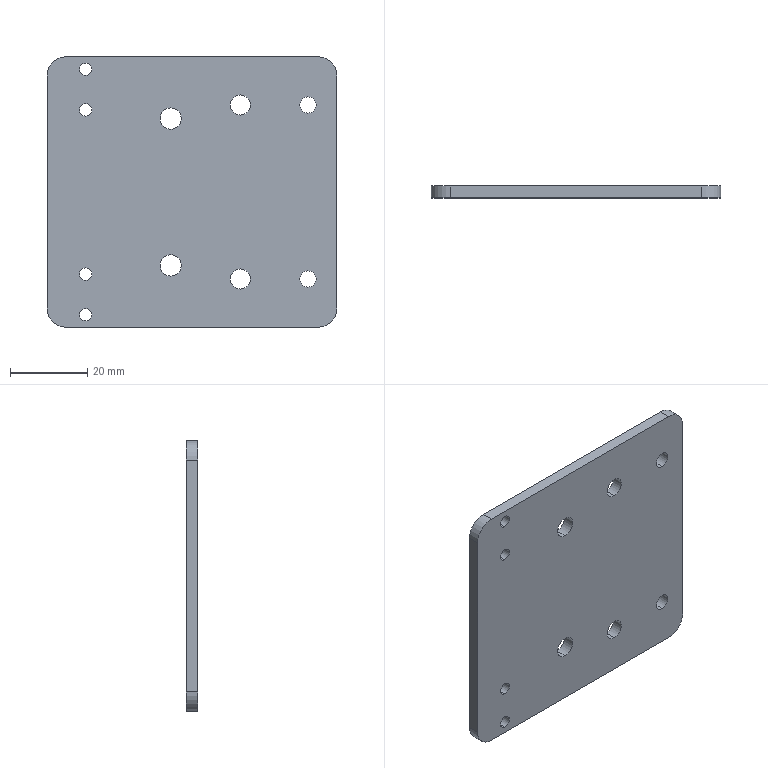Part | SolidWorks | features BaseBody 1 | 1 solid | 30 faces | box 75 x 3 x 70 mm | volume 15236 mm3 | cylinder 24 | plane 6 | commonest cylinder face diameters 3.2 x8 4.2 x4 5.2 x4 5.5 x4 10 x4
STEP:
#1=CARTESIAN_POINT('',(-7.5,3.,25.1));
#2=VERTEX_POINT('',#1);
#3=CARTESIAN_POINT('',(-7.5,3.,19.9));
#4=VERTEX_POINT('',#3);
#5=CARTESIAN_POINT('',(-7.5,3.,22.5));
#6=DIRECTION('',(0.,-1.,0.));
#7=DIRECTION('',(0.,0.,-1.));
#8=AXIS2_PLACEMENT_3D('',#5,#6,#7);
#9=CIRCLE('',#8,2.6);
#10=EDGE_CURVE('',#2,#4,#9,.T.);
#11=ORIENTED_EDGE('',*,*,#10,.F.);
#12=CARTESIAN_POINT('',(-7.5,0.,25.1));
#13=VERTEX_POINT('',#12);
#14=CARTESIAN_POINT('',(-7.5,3.,25.1));
#15=DIRECTION('',(0.,-1.,0.));
#16=VECTOR('',#15,1000.);
#17=LINE('',#14,#16);
#18=EDGE_CURVE('',#2,#13,#17,.T.);
#19=ORIENTED_EDGE('',*,*,#18,.T.);
#20=CARTESIAN_POINT('',(-7.5,0.,19.9));
#21=VERTEX_POINT('',#20);
#22=CARTESIAN_POINT('',(-7.5,0.,22.5));
#23=DIRECTION('',(0.,1.,0.));
#24=DIRECTION('',(0.,0.,-1.));
#25=AXIS2_PLACEMENT_3D('',#22,#23,#24);
#26=CIRCLE('',#25,2.6);
#27=EDGE_CURVE('',#21,#13,#26,.T.);
#28=ORIENTED_EDGE('',*,*,#27,.F.);
#29=CARTESIAN_POINT('',(-7.5,3.,19.9));
#30=DIRECTION('',(0.,-1.,0.));
#31=VECTOR('',#30,1000.);
#32=LINE('',#29,#31);
#33=EDGE_CURVE('',#4,#21,#32,.T.);
#34=ORIENTED_EDGE('',*,*,#33,.F.);
#35=EDGE_LOOP('',(#11,#19,#28,#34));
#36=FACE_OUTER_BOUND('',#35,.T.);
#37=CARTESIAN_POINT('',(-7.5,3.,22.5));
#38=DIRECTION('',(0.,-1.,0.));
#39=DIRECTION('',(0.,0.,-1.));
#40=AXIS2_PLACEMENT_3D('',#37,#38,#39);
#41=CYLINDRICAL_SURFACE('',#40,2.6);
#42=ADVANCED_FACE('',(#36),#41,.F.);
#43=CARTESIAN_POINT('',(-7.5,3.,-19.9));
#44=VERTEX_POINT('',#43);
#45=CARTESIAN_POINT('',(-7.5,3.,-25.1));
#46=VERTEX_POINT('',#45);
#47=CARTESIAN_POINT('',(-7.5,3.,-22.5));
#48=DIRECTION('',(0.,-1.,0.));
#49=DIRECTION('',(0.,0.,-1.));
#50=AXIS2_PLACEMENT_3D('',#47,#48,#49);
#51=CIRCLE('',#50,2.6);
#52=EDGE_CURVE('',#44,#46,#51,.T.);
#53=ORIENTED_EDGE('',*,*,#52,.F.);
#54=CARTESIAN_POINT('',(-7.5,0.,-19.9));
#55=VERTEX_POINT('',#54);
#56=CARTESIAN_POINT('',(-7.5,3.,-19.9));
#57=DIRECTION('',(0.,-1.,0.));
#58=VECTOR('',#57,1000.);
#59=LINE('',#56,#58);
#60=EDGE_CURVE('',#44,#55,#59,.T.);
#61=ORIENTED_EDGE('',*,*,#60,.T.);
#62=CARTESIAN_POINT('',(-7.5,0.,-25.1));
#63=VERTEX_POINT('',#62);
#64=CARTESIAN_POINT('',(-7.5,0.,-22.5));
#65=DIRECTION('',(0.,1.,0.));
#66=DIRECTION('',(0.,0.,-1.));
#67=AXIS2_PLACEMENT_3D('',#64,#65,#66);
#68=CIRCLE('',#67,2.6);
#69=EDGE_CURVE('',#63,#55,#68,.T.);
#70=ORIENTED_EDGE('',*,*,#69,.F.);
#71=CARTESIAN_POINT('',(-7.5,3.,-25.1));
#72=DIRECTION('',(0.,-1.,0.));
#73=VECTOR('',#72,1000.);
#74=LINE('',#71,#73);
#75=EDGE_CURVE('',#46,#63,#74,.T.);
#76=ORIENTED_EDGE('',*,*,#75,.F.);
#77=EDGE_LOOP('',(#53,#61,#70,#76));
#78=FACE_OUTER_BOUND('',#77,.T.);
#79=CARTESIAN_POINT('',(-7.5,3.,-22.5));
#80=DIRECTION('',(0.,-1.,0.));
#81=DIRECTION('',(0.,0.,-1.));
#82=AXIS2_PLACEMENT_3D('',#79,#80,#81);
#83=CYLINDRICAL_SURFACE('',#82,2.6);
#84=ADVANCED_FACE('',(#78),#83,.F.);
#85=CARTESIAN_POINT('',(10.,0.,-24.6));
#86=VERTEX_POINT('',#85);
#87=CARTESIAN_POINT('',(10.,0.,-20.4));
#88=VERTEX_POINT('',#87);
#89=CARTESIAN_POINT('',(10.,0.,-22.5));
#90=DIRECTION('',(0.,1.,0.));
#91=DIRECTION('',(0.,0.,1.));
#92=AXIS2_PLACEMENT_3D('',#89,#90,#91);
#93=CIRCLE('',#92,2.1);
#94=EDGE_CURVE('',#86,#88,#93,.T.);
#95=ORIENTED_EDGE('',*,*,#94,.F.);
#96=CARTESIAN_POINT('',(10.,3.,-24.6));
#97=VERTEX_POINT('',#96);
#98=CARTESIAN_POINT('',(10.,0.,-24.6));
#99=DIRECTION('',(0.,1.,0.));
#100=VECTOR('',#99,1000.);
#101=LINE('',#98,#100);
#102=EDGE_CURVE('',#86,#97,#101,.T.);
#103=ORIENTED_EDGE('',*,*,#102,.T.);
#104=CARTESIAN_POINT('',(10.,3.,-20.4));
#105=VERTEX_POINT('',#104);
#106=CARTESIAN_POINT('',(10.,3.,-22.5));
#107=DIRECTION('',(0.,-1.,0.));
#108=DIRECTION('',(0.,0.,1.));
#109=AXIS2_PLACEMENT_3D('',#106,#107,#108);
#110=CIRCLE('',#109,2.1);
#111=EDGE_CURVE('',#105,#97,#110,.T.);
#112=ORIENTED_EDGE('',*,*,#111,.F.);
#113=CARTESIAN_POINT('',(10.,0.,-20.4));
#114=DIRECTION('',(0.,1.,0.));
#115=VECTOR('',#114,1000.);
#116=LINE('',#113,#115);
#117=EDGE_CURVE('',#88,#105,#116,.T.);
#118=ORIENTED_EDGE('',*,*,#117,.F.);
#119=EDGE_LOOP('',(#95,#103,#112,#118));
#120=FACE_OUTER_BOUND('',#119,.T.);
#121=CARTESIAN_POINT('',(10.,0.,-22.5));
#122=DIRECTION('',(0.,1.,0.));
#123=DIRECTION('',(0.,0.,1.));
#124=AXIS2_PLACEMENT_3D('',#121,#122,#123);
#125=CYLINDRICAL_SURFACE('',#124,2.1);
#126=ADVANCED_FACE('',(#120),#125,.F.);
#127=CARTESIAN_POINT('',(10.,0.,20.4));
#128=VERTEX_POINT('',#127);
#129=CARTESIAN_POINT('',(10.,0.,24.6));
#130=VERTEX_POINT('',#129);
#131=CARTESIAN_POINT('',(10.,0.,22.5));
#132=DIRECTION('',(0.,1.,0.));
#133=DIRECTION('',(0.,0.,1.));
#134=AXIS2_PLACEMENT_3D('',#131,#132,#133);
#135=CIRCLE('',#134,2.1);
#136=EDGE_CURVE('',#128,#130,#135,.T.);
#137=ORIENTED_EDGE('',*,*,#136,.F.);
#138=CARTESIAN_POINT('',(10.,3.,20.4));
#139=VERTEX_POINT('',#138);
#140=CARTESIAN_POINT('',(10.,0.,20.4));
#141=DIRECTION('',(0.,1.,0.));
#142=VECTOR('',#141,1000.);
#143=LINE('',#140,#142);
#144=EDGE_CURVE('',#128,#139,#143,.T.);
#145=ORIENTED_EDGE('',*,*,#144,.T.);
#146=CARTESIAN_POINT('',(10.,3.,24.6));
#147=VERTEX_POINT('',#146);
#148=CARTESIAN_POINT('',(10.,3.,22.5));
#149=DIRECTION('',(0.,-1.,0.));
#150=DIRECTION('',(0.,0.,1.));
#151=AXIS2_PLACEMENT_3D('',#148,#149,#150);
#152=CIRCLE('',#151,2.1);
#153=EDGE_CURVE('',#147,#139,#152,.T.);
#154=ORIENTED_EDGE('',*,*,#153,.F.);
#155=CARTESIAN_POINT('',(10.,0.,24.6));
#156=DIRECTION('',(0.,1.,0.));
#157=VECTOR('',#156,1000.);
#158=LINE('',#155,#157);
#159=EDGE_CURVE('',#130,#147,#158,.T.);
#160=ORIENTED_EDGE('',*,*,#159,.F.);
#161=EDGE_LOOP('',(#137,#145,#154,#160));
#162=FACE_OUTER_BOUND('',#161,.T.);
#163=CARTESIAN_POINT('',(10.,0.,22.5));
#164=DIRECTION('',(0.,1.,0.));
#165=DIRECTION('',(0.,0.,1.));
#166=AXIS2_PLACEMENT_3D('',#163,#164,#165);
#167=CYLINDRICAL_SURFACE('',#166,2.1);
#168=ADVANCED_FACE('',(#162),#167,.F.);
#169=CARTESIAN_POINT('',(-47.5,3.,22.85));
#170=VERTEX_POINT('',#169);
#171=CARTESIAN_POINT('',(-47.5,3.,19.65));
#172=VERTEX_POINT('',#171);
#173=CARTESIAN_POINT('',(-47.5,3.,21.25));
#174=DIRECTION('',(0.,-1.,0.));
#175=DIRECTION('',(0.,0.,-1.));
#176=AXIS2_PLACEMENT_3D('',#173,#174,#175);
#177=CIRCLE('',#176,1.6);
#178=EDGE_CURVE('',#170,#172,#177,.T.);
#179=ORIENTED_EDGE('',*,*,#178,.F.);
#180=CARTESIAN_POINT('',(-47.5,0.,22.85));
#181=VERTEX_POINT('',#180);
#182=CARTESIAN_POINT('',(-47.5,3.,22.85));
#183=DIRECTION('',(0.,-1.,0.));
#184=VECTOR('',#183,1000.);
#185=LINE('',#182,#184);
#186=EDGE_CURVE('',#170,#181,#185,.T.);
#187=ORIENTED_EDGE('',*,*,#186,.T.);
#188=CARTESIAN_POINT('',(-47.5,0.,19.65));
#189=VERTEX_POINT('',#188);
#190=CARTESIAN_POINT('',(-47.5,0.,21.25));
#191=DIRECTION('',(0.,1.,0.));
#192=DIRECTION('',(0.,0.,-1.));
#193=AXIS2_PLACEMENT_3D('',#190,#191,#192);
#194=CIRCLE('',#193,1.6);
#195=EDGE_CURVE('',#189,#181,#194,.T.);
#196=ORIENTED_EDGE('',*,*,#195,.F.);
#197=CARTESIAN_POINT('',(-47.5,3.,19.65));
#198=DIRECTION('',(0.,-1.,0.));
#199=VECTOR('',#198,1000.);
#200=LINE('',#197,#199);
#201=EDGE_CURVE('',#172,#189,#200,.T.);
#202=ORIENTED_EDGE('',*,*,#201,.F.);
#203=EDGE_LOOP('',(#179,#187,#196,#202));
#204=FACE_OUTER_BOUND('',#203,.T.);
#205=CARTESIAN_POINT('',(-47.5,3.,21.25));
#206=DIRECTION('',(0.,-1.,0.));
#207=DIRECTION('',(0.,0.,-1.));
#208=AXIS2_PLACEMENT_3D('',#205,#206,#207);
#209=CYLINDRICAL_SURFACE('',#208,1.6);
#210=ADVANCED_FACE('',(#204),#209,.F.);
#211=CARTESIAN_POINT('',(-47.5,3.,33.35));
#212=VERTEX_POINT('',#211);
#213=CARTESIAN_POINT('',(-47.5,3.,30.15));
#214=VERTEX_POINT('',#213);
#215=CARTESIAN_POINT('',(-47.5,3.,31.75));
#216=DIRECTION('',(0.,-1.,0.));
#217=DIRECTION('',(0.,0.,-1.));
#218=AXIS2_PLACEMENT_3D('',#215,#216,#217);
#219=CIRCLE('',#218,1.6);
#220=EDGE_CURVE('',#212,#214,#219,.T.);
#221=ORIENTED_EDGE('',*,*,#220,.F.);
#222=CARTESIAN_POINT('',(-47.5,0.,33.35));
#223=VERTEX_POINT('',#222);
#224=CARTESIAN_POINT('',(-47.5,3.,33.35));
#225=DIRECTION('',(0.,-1.,0.));
#226=VECTOR('',#225,1000.);
#227=LINE('',#224,#226);
#228=EDGE_CURVE('',#212,#223,#227,.T.);
#229=ORIENTED_EDGE('',*,*,#228,.T.);
#230=CARTESIAN_POINT('',(-47.5,0.,30.15));
#231=VERTEX_POINT('',#230);
#232=CARTESIAN_POINT('',(-47.5,0.,31.75));
#233=DIRECTION('',(0.,1.,0.));
#234=DIRECTION('',(0.,0.,-1.));
#235=AXIS2_PLACEMENT_3D('',#232,#233,#234);
#236=CIRCLE('',#235,1.6);
#237=EDGE_CURVE('',#231,#223,#236,.T.);
#238=ORIENTED_EDGE('',*,*,#237,.F.);
#239=CARTESIAN_POINT('',(-47.5,3.,30.15));
#240=DIRECTION('',(0.,-1.,0.));
#241=VECTOR('',#240,1000.);
#242=LINE('',#239,#241);
#243=EDGE_CURVE('',#214,#231,#242,.T.);
#244=ORIENTED_EDGE('',*,*,#243,.F.);
#245=EDGE_LOOP('',(#221,#229,#238,#244));
#246=FACE_OUTER_BOUND('',#245,.T.);
#247=CARTESIAN_POINT('',(-47.5,3.,31.75));
#248=DIRECTION('',(0.,-1.,0.));
#249=DIRECTION('',(0.,0.,-1.));
#250=AXIS2_PLACEMENT_3D('',#247,#248,#249);
#251=CYLINDRICAL_SURFACE('',#250,1.6);
#252=ADVANCED_FACE('',(#246),#251,.F.);
#253=CARTESIAN_POINT('',(-47.5,3.,-19.65));
#254=VERTEX_POINT('',#253);
#255=CARTESIAN_POINT('',(-47.5,3.,-22.85));
#256=VERTEX_POINT('',#255);
#257=CARTESIAN_POINT('',(-47.5,3.,-21.25));
#258=DIRECTION('',(0.,-1.,0.));
#259=DIRECTION('',(0.,0.,-1.));
#260=AXIS2_PLACEMENT_3D('',#257,#258,#259);
#261=CIRCLE('',#260,1.6);
#262=EDGE_CURVE('',#254,#256,#261,.T.);
#263=ORIENTED_EDGE('',*,*,#262,.F.);
#264=CARTESIAN_POINT('',(-47.5,0.,-19.65));
#265=VERTEX_POINT('',#264);
#266=CARTESIAN_POINT('',(-47.5,3.,-19.65));
#267=DIRECTION('',(0.,-1.,0.));
#268=VECTOR('',#267,1000.);
#269=LINE('',#266,#268);
#270=EDGE_CURVE('',#254,#265,#269,.T.);
#271=ORIENTED_EDGE('',*,*,#270,.T.);
#272=CARTESIAN_POINT('',(-47.5,0.,-22.85));
#273=VERTEX_POINT('',#272);
#274=CARTESIAN_POINT('',(-47.5,0.,-21.25));
#275=DIRECTION('',(0.,1.,0.));
#276=DIRECTION('',(0.,0.,-1.));
#277=AXIS2_PLACEMENT_3D('',#274,#275,#276);
#278=CIRCLE('',#277,1.6);
#279=EDGE_CURVE('',#273,#265,#278,.T.);
#280=ORIENTED_EDGE('',*,*,#279,.F.);
#281=CARTESIAN_POINT('',(-47.5,3.,-22.85));
#282=DIRECTION('',(0.,-1.,0.));
#283=VECTOR('',#282,1000.);
#284=LINE('',#281,#283);
#285=EDGE_CURVE('',#256,#273,#284,.T.);
#286=ORIENTED_EDGE('',*,*,#285,.F.);
#287=EDGE_LOOP('',(#263,#271,#280,#286));
#288=FACE_OUTER_BOUND('',#287,.T.);
#289=CARTESIAN_POINT('',(-47.5,3.,-21.25));
#290=DIRECTION('',(0.,-1.,0.));
#291=DIRECTION('',(0.,0.,-1.));
#292=AXIS2_PLACEMENT_3D('',#289,#290,#291);
#293=CYLINDRICAL_SURFACE('',#292,1.6);
#294=ADVANCED_FACE('',(#288),#293,.F.);
#295=CARTESIAN_POINT('',(-47.5,3.,-30.15));
#296=VERTEX_POINT('',#295);
#297=CARTESIAN_POINT('',(-47.5,3.,-33.35));
#298=VERTEX_POINT('',#297);
#299=CARTESIAN_POINT('',(-47.5,3.,-31.75));
#300=DIRECTION('',(0.,-1.,0.));
#301=DIRECTION('',(0.,0.,-1.));
#302=AXIS2_PLACEMENT_3D('',#299,#300,#301);
#303=CIRCLE('',#302,1.6);
#304=EDGE_CURVE('',#296,#298,#303,.T.);
#305=ORIENTED_EDGE('',*,*,#304,.F.);
#306=CARTESIAN_POINT('',(-47.5,0.,-30.15));
#307=VERTEX_POINT('',#306);
#308=CARTESIAN_POINT('',(-47.5,3.,-30.15));
#309=DIRECTION('',(0.,-1.,0.));
#310=VECTOR('',#309,1000.);
#311=LINE('',#308,#310);
#312=EDGE_CURVE('',#296,#307,#311,.T.);
#313=ORIENTED_EDGE('',*,*,#312,.T.);
#314=CARTESIAN_POINT('',(-47.5,0.,-33.35));
#315=VERTEX_POINT('',#314);
#316=CARTESIAN_POINT('',(-47.5,0.,-31.75));
#317=DIRECTION('',(0.,1.,0.));
#318=DIRECTION('',(0.,0.,-1.));
#319=AXIS2_PLACEMENT_3D('',#316,#317,#318);
#320=CIRCLE('',#319,1.6);
#321=EDGE_CURVE('',#315,#307,#320,.T.);
#322=ORIENTED_EDGE('',*,*,#321,.F.);
#323=CARTESIAN_POINT('',(-47.5,3.,-33.35));
#324=DIRECTION('',(0.,-1.,0.));
#325=VECTOR('',#324,1000.);
#326=LINE('',#323,#325);
#327=EDGE_CURVE('',#298,#315,#326,.T.);
#328=ORIENTED_EDGE('',*,*,#327,.F.);
#329=EDGE_LOOP('',(#305,#313,#322,#328));
#330=FACE_OUTER_BOUND('',#329,.T.);
#331=CARTESIAN_POINT('',(-47.5,3.,-31.75));
#332=DIRECTION('',(0.,-1.,0.));
#333=DIRECTION('',(0.,0.,-1.));
#334=AXIS2_PLACEMENT_3D('',#331,#332,#333);
#335=CYLINDRICAL_SURFACE('',#334,1.6);
#336=ADVANCED_FACE('',(#330),#335,.F.);
#337=CARTESIAN_POINT('',(-25.5,0.,-21.75));
#338=VERTEX_POINT('',#337);
#339=CARTESIAN_POINT('',(-25.5,0.,-16.25));
#340=VERTEX_POINT('',#339);
#341=CARTESIAN_POINT('',(-25.5,0.,-19.));
#342=DIRECTION('',(0.,1.,0.));
#343=DIRECTION('',(0.,0.,1.));
#344=AXIS2_PLACEMENT_3D('',#341,#342,#343);
#345=CIRCLE('',#344,2.75);
#346=EDGE_CURVE('',#338,#340,#345,.T.);
#347=ORIENTED_EDGE('',*,*,#346,.F.);
#348=CARTESIAN_POINT('',(-25.5,3.,-21.75));
#349=VERTEX_POINT('',#348);
#350=CARTESIAN_POINT('',(-25.5,-2.5,-21.75));
#351=DIRECTION('',(0.,1.,0.));
#352=VECTOR('',#351,1000.);
#353=LINE('',#350,#352);
#354=EDGE_CURVE('',#338,#349,#353,.T.);
#355=ORIENTED_EDGE('',*,*,#354,.T.);
#356=CARTESIAN_POINT('',(-25.5,3.,-16.25));
#357=VERTEX_POINT('',#356);
#358=CARTESIAN_POINT('',(-25.5,3.,-19.));
#359=DIRECTION('',(0.,-1.,0.));
#360=DIRECTION('',(0.,0.,1.));
#361=AXIS2_PLACEMENT_3D('',#358,#359,#360);
#362=CIRCLE('',#361,2.75);
#363=EDGE_CURVE('',#357,#349,#362,.T.);
#364=ORIENTED_EDGE('',*,*,#363,.F.);
#365=CARTESIAN_POINT('',(-25.5,-2.5,-16.25));
#366=DIRECTION('',(0.,1.,0.));
#367=VECTOR('',#366,1000.);
#368=LINE('',#365,#367);
#369=EDGE_CURVE('',#340,#357,#368,.T.);
#370=ORIENTED_EDGE('',*,*,#369,.F.);
#371=EDGE_LOOP('',(#347,#355,#364,#370));
#372=FACE_OUTER_BOUND('',#371,.T.);
#373=CARTESIAN_POINT('',(-25.5,-2.5,-19.));
#374=DIRECTION('',(0.,1.,0.));
#375=DIRECTION('',(0.,0.,1.));
#376=AXIS2_PLACEMENT_3D('',#373,#374,#375);
#377=CYLINDRICAL_SURFACE('',#376,2.75);
#378=ADVANCED_FACE('',(#372),#377,.F.);
#379=CARTESIAN_POINT('',(-25.5,0.,16.25));
#380=VERTEX_POINT('',#379);
#381=CARTESIAN_POINT('',(-25.5,0.,21.75));
#382=VERTEX_POINT('',#381);
#383=CARTESIAN_POINT('',(-25.5,0.,19.));
#384=DIRECTION('',(0.,1.,0.));
#385=DIRECTION('',(0.,0.,1.));
#386=AXIS2_PLACEMENT_3D('',#383,#384,#385);
#387=CIRCLE('',#386,2.75);
#388=EDGE_CURVE('',#380,#382,#387,.T.);
#389=ORIENTED_EDGE('',*,*,#388,.F.);
#390=CARTESIAN_POINT('',(-25.5,3.,16.25));
#391=VERTEX_POINT('',#390);
#392=CARTESIAN_POINT('',(-25.5,-2.5,16.25));
#393=DIRECTION('',(0.,1.,0.));
#394=VECTOR('',#393,1000.);
#395=LINE('',#392,#394);
#396=EDGE_CURVE('',#380,#391,#395,.T.);
#397=ORIENTED_EDGE('',*,*,#396,.T.);
#398=CARTESIAN_POINT('',(-25.5,3.,21.75));
#399=VERTEX_POINT('',#398);
#400=CARTESIAN_POINT('',(-25.5,3.,19.));
#401=DIRECTION('',(0.,-1.,0.));
#402=DIRECTION('',(0.,0.,1.));
#403=AXIS2_PLACEMENT_3D('',#400,#401,#402);
#404=CIRCLE('',#403,2.75);
#405=EDGE_CURVE('',#399,#391,#404,.T.);
#406=ORIENTED_EDGE('',*,*,#405,.F.);
#407=CARTESIAN_POINT('',(-25.5,-2.5,21.75));
#408=DIRECTION('',(0.,1.,0.));
#409=VECTOR('',#408,1000.);
#410=LINE('',#407,#409);
#411=EDGE_CURVE('',#382,#399,#410,.T.);
#412=ORIENTED_EDGE('',*,*,#411,.F.);
#413=EDGE_LOOP('',(#389,#397,#406,#412));
#414=FACE_OUTER_BOUND('',#413,.T.);
#415=CARTESIAN_POINT('',(-25.5,-2.5,19.));
#416=DIRECTION('',(0.,1.,0.));
#417=DIRECTION('',(0.,0.,1.));
#418=AXIS2_PLACEMENT_3D('',#415,#416,#417);
#419=CYLINDRICAL_SURFACE('',#418,2.75);
#420=ADVANCED_FACE('',(#414),#419,.F.);
#421=ORIENTED_EDGE('',*,*,#27,.T.);
#422=CARTESIAN_POINT('',(-7.5,0.,22.5));
#423=DIRECTION('',(0.,1.,0.));
#424=DIRECTION('',(0.,0.,-1.));
#425=AXIS2_PLACEMENT_3D('',#422,#423,#424);
#426=CIRCLE('',#425,2.6);
#427=EDGE_CURVE('',#13,#21,#426,.T.);
#428=ORIENTED_EDGE('',*,*,#427,.T.);
#429=EDGE_LOOP('',(#421,#428));
#430=FACE_BOUND('',#429,.T.);
#431=ORIENTED_EDGE('',*,*,#69,.T.);
#432=CARTESIAN_POINT('',(-7.5,0.,-22.5));
#433=DIRECTION('',(0.,1.,0.));
#434=DIRECTION('',(0.,0.,-1.));
#435=AXIS2_PLACEMENT_3D('',#432,#433,#434);
#436=CIRCLE('',#435,2.6);
#437=EDGE_CURVE('',#55,#63,#436,.T.);
#438=ORIENTED_EDGE('',*,*,#437,.T.);
#439=EDGE_LOOP('',(#431,#438));
#440=FACE_BOUND('',#439,.T.);
#441=CARTESIAN_POINT('',(10.,0.,-22.5));
#442=DIRECTION('',(0.,1.,0.));
#443=DIRECTION('',(0.,0.,1.));
#444=AXIS2_PLACEMENT_3D('',#441,#442,#443);
#445=CIRCLE('',#444,2.1);
#446=EDGE_CURVE('',#88,#86,#445,.T.);
#447=ORIENTED_EDGE('',*,*,#446,.T.);
#448=ORIENTED_EDGE('',*,*,#94,.T.);
#449=EDGE_LOOP('',(#447,#448));
#450=FACE_BOUND('',#449,.T.);
#451=CARTESIAN_POINT('',(10.,0.,22.5));
#452=DIRECTION('',(0.,1.,0.));
#453=DIRECTION('',(0.,0.,1.));
#454=AXIS2_PLACEMENT_3D('',#451,#452,#453);
#455=CIRCLE('',#454,2.1);
#456=EDGE_CURVE('',#130,#128,#455,.T.);
#457=ORIENTED_EDGE('',*,*,#456,.T.);
#458=ORIENTED_EDGE('',*,*,#136,.T.);
#459=EDGE_LOOP('',(#457,#458));
#460=FACE_BOUND('',#459,.T.);
#461=ORIENTED_EDGE('',*,*,#195,.T.);
#462=CARTESIAN_POINT('',(-47.5,0.,21.25));
#463=DIRECTION('',(0.,1.,0.));
#464=DIRECTION('',(0.,0.,-1.));
#465=AXIS2_PLACEMENT_3D('',#462,#463,#464);
#466=CIRCLE('',#465,1.6);
#467=EDGE_CURVE('',#181,#189,#466,.T.);
#468=ORIENTED_EDGE('',*,*,#467,.T.);
#469=EDGE_LOOP('',(#461,#468));
#470=FACE_BOUND('',#469,.T.);
#471=ORIENTED_EDGE('',*,*,#237,.T.);
#472=CARTESIAN_POINT('',(-47.5,0.,31.75));
#473=DIRECTION('',(0.,1.,0.));
#474=DIRECTION('',(0.,0.,-1.));
#475=AXIS2_PLACEMENT_3D('',#472,#473,#474);
#476=CIRCLE('',#475,1.6);
#477=EDGE_CURVE('',#223,#231,#476,.T.);
#478=ORIENTED_EDGE('',*,*,#477,.T.);
#479=EDGE_LOOP('',(#471,#478));
#480=FACE_BOUND('',#479,.T.);
#481=ORIENTED_EDGE('',*,*,#279,.T.);
#482=CARTESIAN_POINT('',(-47.5,0.,-21.25));
#483=DIRECTION('',(0.,1.,0.));
#484=DIRECTION('',(0.,0.,-1.));
#485=AXIS2_PLACEMENT_3D('',#482,#483,#484);
#486=CIRCLE('',#485,1.6);
#487=EDGE_CURVE('',#265,#273,#486,.T.);
#488=ORIENTED_EDGE('',*,*,#487,.T.);
#489=EDGE_LOOP('',(#481,#488));
#490=FACE_BOUND('',#489,.T.);
#491=ORIENTED_EDGE('',*,*,#321,.T.);
#492=CARTESIAN_POINT('',(-47.5,0.,-31.75));
#493=DIRECTION('',(0.,1.,0.));
#494=DIRECTION('',(0.,0.,-1.));
#495=AXIS2_PLACEMENT_3D('',#492,#493,#494);
#496=CIRCLE('',#495,1.6);
#497=EDGE_CURVE('',#307,#315,#496,.T.);
#498=ORIENTED_EDGE('',*,*,#497,.T.);
#499=EDGE_LOOP('',(#491,#498));
#500=FACE_BOUND('',#499,.T.);
#501=CARTESIAN_POINT('',(12.5,0.,35.));
#502=VERTEX_POINT('',#501);
#503=CARTESIAN_POINT('',(-52.5,0.,35.));
#504=VERTEX_POINT('',#503);
#505=CARTESIAN_POINT('',(0.,0.,35.));
#506=DIRECTION('',(-1.,0.,0.));
#507=VECTOR('',#506,1000.);
#508=LINE('',#505,#507);
#509=EDGE_CURVE('',#502,#504,#508,.T.);
#510=ORIENTED_EDGE('',*,*,#509,.T.);
#511=CARTESIAN_POINT('',(-57.5,0.,30.));
#512=VERTEX_POINT('',#511);
#513=CARTESIAN_POINT('',(-52.5,0.,30.));
#514=DIRECTION('',(0.,-1.,0.));
#515=DIRECTION('',(0.,0.,1.));
#516=AXIS2_PLACEMENT_3D('',#513,#514,#515);
#517=CIRCLE('',#516,5.);
#518=EDGE_CURVE('',#504,#512,#517,.T.);
#519=ORIENTED_EDGE('',*,*,#518,.T.);
#520=CARTESIAN_POINT('',(-57.5,0.,-30.));
#521=VERTEX_POINT('',#520);
#522=CARTESIAN_POINT('',(-57.5,0.,0.));
#523=DIRECTION('',(0.,0.,-1.));
#524=VECTOR('',#523,1000.);
#525=LINE('',#522,#524);
#526=EDGE_CURVE('',#512,#521,#525,.T.);
#527=ORIENTED_EDGE('',*,*,#526,.T.);
#528=CARTESIAN_POINT('',(-52.5,0.,-35.));
#529=VERTEX_POINT('',#528);
#530=CARTESIAN_POINT('',(-52.5,0.,-30.));
#531=DIRECTION('',(0.,-1.,0.));
#532=DIRECTION('',(0.,0.,1.));
#533=AXIS2_PLACEMENT_3D('',#530,#531,#532);
#534=CIRCLE('',#533,5.);
#535=EDGE_CURVE('',#521,#529,#534,.T.);
#536=ORIENTED_EDGE('',*,*,#535,.T.);
#537=CARTESIAN_POINT('',(12.5,0.,-35.));
#538=VERTEX_POINT('',#537);
#539=CARTESIAN_POINT('',(0.,0.,-35.));
#540=DIRECTION('',(1.,0.,0.));
#541=VECTOR('',#540,1000.);
#542=LINE('',#539,#541);
#543=EDGE_CURVE('',#529,#538,#542,.T.);
#544=ORIENTED_EDGE('',*,*,#543,.T.);
#545=CARTESIAN_POINT('',(17.5,0.,-30.));
#546=VERTEX_POINT('',#545);
#547=CARTESIAN_POINT('',(12.5,0.,-30.));
#548=DIRECTION('',(0.,-1.,0.));
#549=DIRECTION('',(0.,0.,-1.));
#550=AXIS2_PLACEMENT_3D('',#547,#548,#549);
#551=CIRCLE('',#550,5.);
#552=EDGE_CURVE('',#538,#546,#551,.T.);
#553=ORIENTED_EDGE('',*,*,#552,.T.);
#554=CARTESIAN_POINT('',(17.5,0.,30.));
#555=VERTEX_POINT('',#554);
#556=CARTESIAN_POINT('',(17.5,0.,0.));
#557=DIRECTION('',(0.,0.,1.));
#558=VECTOR('',#557,1000.);
#559=LINE('',#556,#558);
#560=EDGE_CURVE('',#546,#555,#559,.T.);
#561=ORIENTED_EDGE('',*,*,#560,.T.);
#562=CARTESIAN_POINT('',(12.5,0.,30.));
#563=DIRECTION('',(0.,-1.,0.));
#564=DIRECTION('',(0.,0.,-1.));
#565=AXIS2_PLACEMENT_3D('',#562,#563,#564);
#566=CIRCLE('',#565,5.);
#567=EDGE_CURVE('',#555,#502,#566,.T.);
#568=ORIENTED_EDGE('',*,*,#567,.T.);
#569=EDGE_LOOP('',(#510,#519,#527,#536,#544,#553,#561,#568));
#570=FACE_OUTER_BOUND('',#569,.T.);
#571=CARTESIAN_POINT('',(-25.5,0.,-19.));
#572=DIRECTION('',(0.,1.,0.));
#573=DIRECTION('',(0.,0.,1.));
#574=AXIS2_PLACEMENT_3D('',#571,#572,#573);
#575=CIRCLE('',#574,2.75);
#576=EDGE_CURVE('',#340,#338,#575,.T.);
#577=ORIENTED_EDGE('',*,*,#576,.T.);
#578=ORIENTED_EDGE('',*,*,#346,.T.);
#579=EDGE_LOOP('',(#577,#578));
#580=FACE_BOUND('',#579,.T.);
#581=CARTESIAN_POINT('',(-25.5,0.,19.));
#582=DIRECTION('',(0.,1.,0.));
#583=DIRECTION('',(0.,0.,1.));
#584=AXIS2_PLACEMENT_3D('',#581,#582,#583);
#585=CIRCLE('',#584,2.75);
#586=EDGE_CURVE('',#382,#380,#585,.T.);
#587=ORIENTED_EDGE('',*,*,#586,.T.);
#588=ORIENTED_EDGE('',*,*,#388,.T.);
#589=EDGE_LOOP('',(#587,#588));
#590=FACE_BOUND('',#589,.T.);
#591=CARTESIAN_POINT('',(0.,0.,0.));
#592=DIRECTION('',(0.,-1.,0.));
#593=DIRECTION('',(0.,0.,-1.));
#594=AXIS2_PLACEMENT_3D('',#591,#592,#593);
#595=PLANE('',#594);
#596=ADVANCED_FACE('',(#430,#440,#450,#460,#470,#480,#490,#500,#570,#580,#590),#595,.T.);
#597=ORIENTED_EDGE('',*,*,#18,.F.);
#598=CARTESIAN_POINT('',(-7.5,3.,22.5));
#599=DIRECTION('',(0.,-1.,0.));
#600=DIRECTION('',(0.,0.,-1.));
#601=AXIS2_PLACEMENT_3D('',#598,#599,#600);
#602=CIRCLE('',#601,2.6);
#603=EDGE_CURVE('',#4,#2,#602,.T.);
#604=ORIENTED_EDGE('',*,*,#603,.F.);
#605=ORIENTED_EDGE('',*,*,#33,.T.);
#606=ORIENTED_EDGE('',*,*,#427,.F.);
#607=EDGE_LOOP('',(#597,#604,#605,#606));
#608=FACE_OUTER_BOUND('',#607,.T.);
#609=CARTESIAN_POINT('',(-7.5,3.,22.5));
#610=DIRECTION('',(0.,-1.,0.));
#611=DIRECTION('',(0.,0.,-1.));
#612=AXIS2_PLACEMENT_3D('',#609,#610,#611);
#613=CYLINDRICAL_SURFACE('',#612,2.6);
#614=ADVANCED_FACE('',(#608),#613,.F.);
#615=ORIENTED_EDGE('',*,*,#60,.F.);
#616=CARTESIAN_POINT('',(-7.5,3.,-22.5));
#617=DIRECTION('',(0.,-1.,0.));
#618=DIRECTION('',(0.,0.,-1.));
#619=AXIS2_PLACEMENT_3D('',#616,#617,#618);
#620=CIRCLE('',#619,2.6);
#621=EDGE_CURVE('',#46,#44,#620,.T.);
#622=ORIENTED_EDGE('',*,*,#621,.F.);
#623=ORIENTED_EDGE('',*,*,#75,.T.);
#624=ORIENTED_EDGE('',*,*,#437,.F.);
#625=EDGE_LOOP('',(#615,#622,#623,#624));
#626=FACE_OUTER_BOUND('',#625,.T.);
#627=CARTESIAN_POINT('',(-7.5,3.,-22.5));
#628=DIRECTION('',(0.,-1.,0.));
#629=DIRECTION('',(0.,0.,-1.));
#630=AXIS2_PLACEMENT_3D('',#627,#628,#629);
#631=CYLINDRICAL_SURFACE('',#630,2.6);
#632=ADVANCED_FACE('',(#626),#631,.F.);
#633=ORIENTED_EDGE('',*,*,#102,.F.);
#634=ORIENTED_EDGE('',*,*,#446,.F.);
#635=ORIENTED_EDGE('',*,*,#117,.T.);
#636=CARTESIAN_POINT('',(10.,3.,-22.5));
#637=DIRECTION('',(0.,-1.,0.));
#638=DIRECTION('',(0.,0.,1.));
#639=AXIS2_PLACEMENT_3D('',#636,#637,#638);
#640=CIRCLE('',#639,2.1);
#641=EDGE_CURVE('',#97,#105,#640,.T.);
#642=ORIENTED_EDGE('',*,*,#641,.F.);
#643=EDGE_LOOP('',(#633,#634,#635,#642));
#644=FACE_OUTER_BOUND('',#643,.T.);
#645=CARTESIAN_POINT('',(10.,0.,-22.5));
#646=DIRECTION('',(0.,1.,0.));
#647=DIRECTION('',(0.,0.,1.));
#648=AXIS2_PLACEMENT_3D('',#645,#646,#647);
#649=CYLINDRICAL_SURFACE('',#648,2.1);
#650=ADVANCED_FACE('',(#644),#649,.F.);
#651=ORIENTED_EDGE('',*,*,#144,.F.);
#652=ORIENTED_EDGE('',*,*,#456,.F.);
#653=ORIENTED_EDGE('',*,*,#159,.T.);
#654=CARTESIAN_POINT('',(10.,3.,22.5));
#655=DIRECTION('',(0.,-1.,0.));
#656=DIRECTION('',(0.,0.,1.));
#657=AXIS2_PLACEMENT_3D('',#654,#655,#656);
#658=CIRCLE('',#657,2.1);
#659=EDGE_CURVE('',#139,#147,#658,.T.);
#660=ORIENTED_EDGE('',*,*,#659,.F.);
#661=EDGE_LOOP('',(#651,#652,#653,#660));
#662=FACE_OUTER_BOUND('',#661,.T.);
#663=CARTESIAN_POINT('',(10.,0.,22.5));
#664=DIRECTION('',(0.,1.,0.));
#665=DIRECTION('',(0.,0.,1.));
#666=AXIS2_PLACEMENT_3D('',#663,#664,#665);
#667=CYLINDRICAL_SURFACE('',#666,2.1);
#668=ADVANCED_FACE('',(#662),#667,.F.);
#669=ORIENTED_EDGE('',*,*,#186,.F.);
#670=CARTESIAN_POINT('',(-47.5,3.,21.25));
#671=DIRECTION('',(0.,-1.,0.));
#672=DIRECTION('',(0.,0.,-1.));
#673=AXIS2_PLACEMENT_3D('',#670,#671,#672);
#674=CIRCLE('',#673,1.6);
#675=EDGE_CURVE('',#172,#170,#674,.T.);
#676=ORIENTED_EDGE('',*,*,#675,.F.);
#677=ORIENTED_EDGE('',*,*,#201,.T.);
#678=ORIENTED_EDGE('',*,*,#467,.F.);
#679=EDGE_LOOP('',(#669,#676,#677,#678));
#680=FACE_OUTER_BOUND('',#679,.T.);
#681=CARTESIAN_POINT('',(-47.5,3.,21.25));
#682=DIRECTION('',(0.,-1.,0.));
#683=DIRECTION('',(0.,0.,-1.));
#684=AXIS2_PLACEMENT_3D('',#681,#682,#683);
#685=CYLINDRICAL_SURFACE('',#684,1.6);
#686=ADVANCED_FACE('',(#680),#685,.F.);
#687=ORIENTED_EDGE('',*,*,#228,.F.);
#688=CARTESIAN_POINT('',(-47.5,3.,31.75));
#689=DIRECTION('',(0.,-1.,0.));
#690=DIRECTION('',(0.,0.,-1.));
#691=AXIS2_PLACEMENT_3D('',#688,#689,#690);
#692=CIRCLE('',#691,1.6);
#693=EDGE_CURVE('',#214,#212,#692,.T.);
#694=ORIENTED_EDGE('',*,*,#693,.F.);
#695=ORIENTED_EDGE('',*,*,#243,.T.);
#696=ORIENTED_EDGE('',*,*,#477,.F.);
#697=EDGE_LOOP('',(#687,#694,#695,#696));
#698=FACE_OUTER_BOUND('',#697,.T.);
#699=CARTESIAN_POINT('',(-47.5,3.,31.75));
#700=DIRECTION('',(0.,-1.,0.));
#701=DIRECTION('',(0.,0.,-1.));
#702=AXIS2_PLACEMENT_3D('',#699,#700,#701);
#703=CYLINDRICAL_SURFACE('',#702,1.6);
#704=ADVANCED_FACE('',(#698),#703,.F.);
#705=ORIENTED_EDGE('',*,*,#270,.F.);
#706=CARTESIAN_POINT('',(-47.5,3.,-21.25));
#707=DIRECTION('',(0.,-1.,0.));
#708=DIRECTION('',(0.,0.,-1.));
#709=AXIS2_PLACEMENT_3D('',#706,#707,#708);
#710=CIRCLE('',#709,1.6);
#711=EDGE_CURVE('',#256,#254,#710,.T.);
#712=ORIENTED_EDGE('',*,*,#711,.F.);
#713=ORIENTED_EDGE('',*,*,#285,.T.);
#714=ORIENTED_EDGE('',*,*,#487,.F.);
#715=EDGE_LOOP('',(#705,#712,#713,#714));
#716=FACE_OUTER_BOUND('',#715,.T.);
#717=CARTESIAN_POINT('',(-47.5,3.,-21.25));
#718=DIRECTION('',(0.,-1.,0.));
#719=DIRECTION('',(0.,0.,-1.));
#720=AXIS2_PLACEMENT_3D('',#717,#718,#719);
#721=CYLINDRICAL_SURFACE('',#720,1.6);
#722=ADVANCED_FACE('',(#716),#721,.F.);
#723=ORIENTED_EDGE('',*,*,#312,.F.);
#724=CARTESIAN_POINT('',(-47.5,3.,-31.75));
#725=DIRECTION('',(0.,-1.,0.));
#726=DIRECTION('',(0.,0.,-1.));
#727=AXIS2_PLACEMENT_3D('',#724,#725,#726);
#728=CIRCLE('',#727,1.6);
#729=EDGE_CURVE('',#298,#296,#728,.T.);
#730=ORIENTED_EDGE('',*,*,#729,.F.);
#731=ORIENTED_EDGE('',*,*,#327,.T.);
#732=ORIENTED_EDGE('',*,*,#497,.F.);
#733=EDGE_LOOP('',(#723,#730,#731,#732));
#734=FACE_OUTER_BOUND('',#733,.T.);
#735=CARTESIAN_POINT('',(-47.5,3.,-31.75));
#736=DIRECTION('',(0.,-1.,0.));
#737=DIRECTION('',(0.,0.,-1.));
#738=AXIS2_PLACEMENT_3D('',#735,#736,#737);
#739=CYLINDRICAL_SURFACE('',#738,1.6);
#740=ADVANCED_FACE('',(#734),#739,.F.);
#741=CARTESIAN_POINT('',(-52.5,3.,35.));
#742=VERTEX_POINT('',#741);
#743=CARTESIAN_POINT('',(-57.5,3.,30.));
#744=VERTEX_POINT('',#743);
#745=CARTESIAN_POINT('',(-52.5,3.,30.));
#746=DIRECTION('',(0.,-1.,0.));
#747=DIRECTION('',(0.,0.,1.));
#748=AXIS2_PLACEMENT_3D('',#745,#746,#747);
#749=CIRCLE('',#748,5.);
#750=EDGE_CURVE('',#742,#744,#749,.T.);
#751=ORIENTED_EDGE('',*,*,#750,.T.);
#752=CARTESIAN_POINT('',(-57.5,-53.,30.));
#753=DIRECTION('',(0.,-1.,0.));
#754=VECTOR('',#753,1000.);
#755=LINE('',#752,#754);
#756=EDGE_CURVE('',#744,#512,#755,.T.);
#757=ORIENTED_EDGE('',*,*,#756,.T.);
#758=ORIENTED_EDGE('',*,*,#518,.F.);
#759=CARTESIAN_POINT('',(-52.5,-53.,35.));
#760=DIRECTION('',(0.,1.,0.));
#761=VECTOR('',#760,1000.);
#762=LINE('',#759,#761);
#763=EDGE_CURVE('',#504,#742,#762,.T.);
#764=ORIENTED_EDGE('',*,*,#763,.T.);
#765=EDGE_LOOP('',(#751,#757,#758,#764));
#766=FACE_OUTER_BOUND('',#765,.T.);
#767=CARTESIAN_POINT('',(-52.5,-53.,30.));
#768=DIRECTION('',(0.,1.,0.));
#769=DIRECTION('',(0.,0.,1.));
#770=AXIS2_PLACEMENT_3D('',#767,#768,#769);
#771=CYLINDRICAL_SURFACE('',#770,5.);
#772=ADVANCED_FACE('',(#766),#771,.T.);
#773=ORIENTED_EDGE('',*,*,#763,.F.);
#774=ORIENTED_EDGE('',*,*,#509,.F.);
#775=CARTESIAN_POINT('',(12.5,3.,35.));
#776=VERTEX_POINT('',#775);
#777=CARTESIAN_POINT('',(12.5,3.,35.));
#778=DIRECTION('',(0.,-1.,0.));
#779=VECTOR('',#778,1000.);
#780=LINE('',#777,#779);
#781=EDGE_CURVE('',#776,#502,#780,.T.);
#782=ORIENTED_EDGE('',*,*,#781,.F.);
#783=CARTESIAN_POINT('',(-17.5,3.,35.));
#784=DIRECTION('',(1.,0.,0.));
#785=VECTOR('',#784,1000.);
#786=LINE('',#783,#785);
#787=EDGE_CURVE('',#742,#776,#786,.T.);
#788=ORIENTED_EDGE('',*,*,#787,.F.);
#789=EDGE_LOOP('',(#773,#774,#782,#788));
#790=FACE_OUTER_BOUND('',#789,.T.);
#791=CARTESIAN_POINT('',(-17.5,3.,35.));
#792=DIRECTION('',(0.,0.,-1.));
#793=DIRECTION('',(-1.,0.,0.));
#794=AXIS2_PLACEMENT_3D('',#791,#792,#793);
#795=PLANE('',#794);
#796=ADVANCED_FACE('',(#790),#795,.F.);
#797=ORIENTED_EDGE('',*,*,#567,.F.);
#798=CARTESIAN_POINT('',(17.5,3.,30.));
#799=VERTEX_POINT('',#798);
#800=CARTESIAN_POINT('',(17.5,3.,30.));
#801=DIRECTION('',(0.,1.,0.));
#802=VECTOR('',#801,1000.);
#803=LINE('',#800,#802);
#804=EDGE_CURVE('',#555,#799,#803,.T.);
#805=ORIENTED_EDGE('',*,*,#804,.T.);
#806=CARTESIAN_POINT('',(12.5,3.,30.));
#807=DIRECTION('',(0.,-1.,0.));
#808=DIRECTION('',(0.,0.,-1.));
#809=AXIS2_PLACEMENT_3D('',#806,#807,#808);
#810=CIRCLE('',#809,5.);
#811=EDGE_CURVE('',#799,#776,#810,.T.);
#812=ORIENTED_EDGE('',*,*,#811,.T.);
#813=ORIENTED_EDGE('',*,*,#781,.T.);
#814=EDGE_LOOP('',(#797,#805,#812,#813));
#815=FACE_OUTER_BOUND('',#814,.T.);
#816=CARTESIAN_POINT('',(12.5,3.,30.));
#817=DIRECTION('',(0.,-1.,0.));
#818=DIRECTION('',(0.,0.,-1.));
#819=AXIS2_PLACEMENT_3D('',#816,#817,#818);
#820=CYLINDRICAL_SURFACE('',#819,5.);
#821=ADVANCED_FACE('',(#815),#820,.T.);
#822=CARTESIAN_POINT('',(17.5,3.,-30.));
#823=VERTEX_POINT('',#822);
#824=CARTESIAN_POINT('',(17.5,3.,-30.));
#825=DIRECTION('',(0.,-1.,0.));
#826=VECTOR('',#825,1000.);
#827=LINE('',#824,#826);
#828=EDGE_CURVE('',#823,#546,#827,.T.);
#829=ORIENTED_EDGE('',*,*,#828,.F.);
#830=CARTESIAN_POINT('',(17.5,3.,35.));
#831=DIRECTION('',(0.,0.,-1.));
#832=VECTOR('',#831,1000.);
#833=LINE('',#830,#832);
#834=EDGE_CURVE('',#799,#823,#833,.T.);
#835=ORIENTED_EDGE('',*,*,#834,.F.);
#836=ORIENTED_EDGE('',*,*,#804,.F.);
#837=ORIENTED_EDGE('',*,*,#560,.F.);
#838=EDGE_LOOP('',(#829,#835,#836,#837));
#839=FACE_OUTER_BOUND('',#838,.T.);
#840=CARTESIAN_POINT('',(17.5,3.,35.));
#841=DIRECTION('',(-1.,0.,0.));
#842=DIRECTION('',(0.,0.,1.));
#843=AXIS2_PLACEMENT_3D('',#840,#841,#842);
#844=PLANE('',#843);
#845=ADVANCED_FACE('',(#839),#844,.F.);
#846=ORIENTED_EDGE('',*,*,#552,.F.);
#847=CARTESIAN_POINT('',(12.5,3.,-35.));
#848=VERTEX_POINT('',#847);
#849=CARTESIAN_POINT('',(12.5,3.,-35.));
#850=DIRECTION('',(0.,1.,0.));
#851=VECTOR('',#850,1000.);
#852=LINE('',#849,#851);
#853=EDGE_CURVE('',#538,#848,#852,.T.);
#854=ORIENTED_EDGE('',*,*,#853,.T.);
#855=CARTESIAN_POINT('',(12.5,3.,-30.));
#856=DIRECTION('',(0.,-1.,0.));
#857=DIRECTION('',(0.,0.,-1.));
#858=AXIS2_PLACEMENT_3D('',#855,#856,#857);
#859=CIRCLE('',#858,5.);
#860=EDGE_CURVE('',#848,#823,#859,.T.);
#861=ORIENTED_EDGE('',*,*,#860,.T.);
#862=ORIENTED_EDGE('',*,*,#828,.T.);
#863=EDGE_LOOP('',(#846,#854,#861,#862));
#864=FACE_OUTER_BOUND('',#863,.T.);
#865=CARTESIAN_POINT('',(12.5,3.,-30.));
#866=DIRECTION('',(0.,-1.,0.));
#867=DIRECTION('',(0.,0.,-1.));
#868=AXIS2_PLACEMENT_3D('',#865,#866,#867);
#869=CYLINDRICAL_SURFACE('',#868,5.);
#870=ADVANCED_FACE('',(#864),#869,.T.);
#871=CARTESIAN_POINT('',(-52.5,3.,-35.));
#872=VERTEX_POINT('',#871);
#873=CARTESIAN_POINT('',(-52.5,3.,-35.));
#874=DIRECTION('',(0.,-1.,0.));
#875=VECTOR('',#874,1000.);
#876=LINE('',#873,#875);
#877=EDGE_CURVE('',#872,#529,#876,.T.);
#878=ORIENTED_EDGE('',*,*,#877,.F.);
#879=CARTESIAN_POINT('',(-17.5,3.,-35.));
#880=DIRECTION('',(-1.,0.,0.));
#881=VECTOR('',#880,1000.);
#882=LINE('',#879,#881);
#883=EDGE_CURVE('',#848,#872,#882,.T.);
#884=ORIENTED_EDGE('',*,*,#883,.F.);
#885=ORIENTED_EDGE('',*,*,#853,.F.);
#886=ORIENTED_EDGE('',*,*,#543,.F.);
#887=EDGE_LOOP('',(#878,#884,#885,#886));
#888=FACE_OUTER_BOUND('',#887,.T.);
#889=CARTESIAN_POINT('',(-17.5,3.,-35.));
#890=DIRECTION('',(0.,0.,1.));
#891=DIRECTION('',(1.,0.,0.));
#892=AXIS2_PLACEMENT_3D('',#889,#890,#891);
#893=PLANE('',#892);
#894=ADVANCED_FACE('',(#888),#893,.F.);
#895=CARTESIAN_POINT('',(-57.5,3.,-30.));
#896=VERTEX_POINT('',#895);
#897=CARTESIAN_POINT('',(-52.5,3.,-30.));
#898=DIRECTION('',(0.,-1.,0.));
#899=DIRECTION('',(0.,0.,1.));
#900=AXIS2_PLACEMENT_3D('',#897,#898,#899);
#901=CIRCLE('',#900,5.);
#902=EDGE_CURVE('',#896,#872,#901,.T.);
#903=ORIENTED_EDGE('',*,*,#902,.T.);
#904=ORIENTED_EDGE('',*,*,#877,.T.);
#905=ORIENTED_EDGE('',*,*,#535,.F.);
#906=CARTESIAN_POINT('',(-57.5,3.,-30.));
#907=DIRECTION('',(0.,1.,0.));
#908=VECTOR('',#907,1000.);
#909=LINE('',#906,#908);
#910=EDGE_CURVE('',#521,#896,#909,.T.);
#911=ORIENTED_EDGE('',*,*,#910,.T.);
#912=EDGE_LOOP('',(#903,#904,#905,#911));
#913=FACE_OUTER_BOUND('',#912,.T.);
#914=CARTESIAN_POINT('',(-52.5,3.,-30.));
#915=DIRECTION('',(0.,1.,0.));
#916=DIRECTION('',(0.,0.,1.));
#917=AXIS2_PLACEMENT_3D('',#914,#915,#916);
#918=CYLINDRICAL_SURFACE('',#917,5.);
#919=ADVANCED_FACE('',(#913),#918,.T.);
#920=ORIENTED_EDGE('',*,*,#910,.F.);
#921=ORIENTED_EDGE('',*,*,#526,.F.);
#922=ORIENTED_EDGE('',*,*,#756,.F.);
#923=CARTESIAN_POINT('',(-57.5,3.,35.));
#924=DIRECTION('',(0.,0.,1.));
#925=VECTOR('',#924,1000.);
#926=LINE('',#923,#925);
#927=EDGE_CURVE('',#896,#744,#926,.T.);
#928=ORIENTED_EDGE('',*,*,#927,.F.);
#929=EDGE_LOOP('',(#920,#921,#922,#928));
#930=FACE_OUTER_BOUND('',#929,.T.);
#931=CARTESIAN_POINT('',(-57.5,-53.,35.));
#932=DIRECTION('',(1.,0.,0.));
#933=DIRECTION('',(0.,0.,-1.));
#934=AXIS2_PLACEMENT_3D('',#931,#932,#933);
#935=PLANE('',#934);
#936=ADVANCED_FACE('',(#930),#935,.F.);
#937=ORIENTED_EDGE('',*,*,#354,.F.);
#938=ORIENTED_EDGE('',*,*,#576,.F.);
#939=ORIENTED_EDGE('',*,*,#369,.T.);
#940=CARTESIAN_POINT('',(-25.5,3.,-19.));
#941=DIRECTION('',(0.,-1.,0.));
#942=DIRECTION('',(0.,0.,1.));
#943=AXIS2_PLACEMENT_3D('',#940,#941,#942);
#944=CIRCLE('',#943,2.75);
#945=EDGE_CURVE('',#349,#357,#944,.T.);
#946=ORIENTED_EDGE('',*,*,#945,.F.);
#947=EDGE_LOOP('',(#937,#938,#939,#946));
#948=FACE_OUTER_BOUND('',#947,.T.);
#949=CARTESIAN_POINT('',(-25.5,-2.5,-19.));
#950=DIRECTION('',(0.,1.,0.));
#951=DIRECTION('',(0.,0.,1.));
#952=AXIS2_PLACEMENT_3D('',#949,#950,#951);
#953=CYLINDRICAL_SURFACE('',#952,2.75);
#954=ADVANCED_FACE('',(#948),#953,.F.);
#955=ORIENTED_EDGE('',*,*,#396,.F.);
#956=ORIENTED_EDGE('',*,*,#586,.F.);
#957=ORIENTED_EDGE('',*,*,#411,.T.);
#958=CARTESIAN_POINT('',(-25.5,3.,19.));
#959=DIRECTION('',(0.,-1.,0.));
#960=DIRECTION('',(0.,0.,1.));
#961=AXIS2_PLACEMENT_3D('',#958,#959,#960);
#962=CIRCLE('',#961,2.75);
#963=EDGE_CURVE('',#391,#399,#962,.T.);
#964=ORIENTED_EDGE('',*,*,#963,.F.);
#965=EDGE_LOOP('',(#955,#956,#957,#964));
#966=FACE_OUTER_BOUND('',#965,.T.);
#967=CARTESIAN_POINT('',(-25.5,-2.5,19.));
#968=DIRECTION('',(0.,1.,0.));
#969=DIRECTION('',(0.,0.,1.));
#970=AXIS2_PLACEMENT_3D('',#967,#968,#969);
#971=CYLINDRICAL_SURFACE('',#970,2.75);
#972=ADVANCED_FACE('',(#966),#971,.F.);
#973=ORIENTED_EDGE('',*,*,#603,.T.);
#974=ORIENTED_EDGE('',*,*,#10,.T.);
#975=EDGE_LOOP('',(#973,#974));
#976=FACE_BOUND('',#975,.T.);
#977=ORIENTED_EDGE('',*,*,#621,.T.);
#978=ORIENTED_EDGE('',*,*,#52,.T.);
#979=EDGE_LOOP('',(#977,#978));
#980=FACE_BOUND('',#979,.T.);
#981=ORIENTED_EDGE('',*,*,#902,.F.);
#982=ORIENTED_EDGE('',*,*,#927,.T.);
#983=ORIENTED_EDGE('',*,*,#750,.F.);
#984=ORIENTED_EDGE('',*,*,#787,.T.);
#985=ORIENTED_EDGE('',*,*,#811,.F.);
#986=ORIENTED_EDGE('',*,*,#834,.T.);
#987=ORIENTED_EDGE('',*,*,#860,.F.);
#988=ORIENTED_EDGE('',*,*,#883,.T.);
#989=EDGE_LOOP('',(#981,#982,#983,#984,#985,#986,#987,#988));
#990=FACE_OUTER_BOUND('',#989,.T.);
#991=ORIENTED_EDGE('',*,*,#111,.T.);
#992=ORIENTED_EDGE('',*,*,#641,.T.);
#993=EDGE_LOOP('',(#991,#992));
#994=FACE_BOUND('',#993,.T.);
#995=ORIENTED_EDGE('',*,*,#153,.T.);
#996=ORIENTED_EDGE('',*,*,#659,.T.);
#997=EDGE_LOOP('',(#995,#996));
#998=FACE_BOUND('',#997,.T.);
#999=ORIENTED_EDGE('',*,*,#675,.T.);
#1000=ORIENTED_EDGE('',*,*,#178,.T.);
#1001=EDGE_LOOP('',(#999,#1000));
#1002=FACE_BOUND('',#1001,.T.);
#1003=ORIENTED_EDGE('',*,*,#693,.T.);
#1004=ORIENTED_EDGE('',*,*,#220,.T.);
#1005=EDGE_LOOP('',(#1003,#1004));
#1006=FACE_BOUND('',#1005,.T.);
#1007=ORIENTED_EDGE('',*,*,#711,.T.);
#1008=ORIENTED_EDGE('',*,*,#262,.T.);
#1009=EDGE_LOOP('',(#1007,#1008));
#1010=FACE_BOUND('',#1009,.T.);
#1011=ORIENTED_EDGE('',*,*,#729,.T.);
#1012=ORIENTED_EDGE('',*,*,#304,.T.);
#1013=EDGE_LOOP('',(#1011,#1012));
#1014=FACE_BOUND('',#1013,.T.);
#1015=ORIENTED_EDGE('',*,*,#363,.T.);
#1016=ORIENTED_EDGE('',*,*,#945,.T.);
#1017=EDGE_LOOP('',(#1015,#1016));
#1018=FACE_BOUND('',#1017,.T.);
#1019=ORIENTED_EDGE('',*,*,#405,.T.);
#1020=ORIENTED_EDGE('',*,*,#963,.T.);
#1021=EDGE_LOOP('',(#1019,#1020));
#1022=FACE_BOUND('',#1021,.T.);
#1023=CARTESIAN_POINT('',(0.,3.,0.));
#1024=DIRECTION('',(0.,-1.,0.));
#1025=DIRECTION('',(0.,0.,-1.));
#1026=AXIS2_PLACEMENT_3D('',#1023,#1024,#1025);
#1027=PLANE('',#1026);
#1028=ADVANCED_FACE('',(#976,#980,#990,#994,#998,#1002,#1006,#1010,#1014,#1018,#1022),#1027,.F.);
#1029=CLOSED_SHELL('',(#42,#84,#126,#168,#210,#252,#294,#336,#378,#420,#596,#614,#632,#650,#668,#686,#704,#722,#740,#772,#796,#821,#845,#870,#894,#919,#936,#954,#972,#1028));
#1030=MANIFOLD_SOLID_BREP('',#1029);
#1031=CARTESIAN_POINT('',(0.,0.,0.));
#1032=DIRECTION('',(0.,0.,1.));
#1033=DIRECTION('',(1.,0.,0.));
#1034=AXIS2_PLACEMENT_3D('',#1031,#1032,#1033);
#1035=(LENGTH_UNIT()NAMED_UNIT(*)SI_UNIT(.MILLI.,.METRE.));
#1036=UNCERTAINTY_MEASURE_WITH_UNIT(LENGTH_MEASURE(0.00001),#1035,'','');
#1037=(NAMED_UNIT(*)PLANE_ANGLE_UNIT()SI_UNIT($,.RADIAN.));
#1038=(NAMED_UNIT(*)SI_UNIT($,.STERADIAN.)SOLID_ANGLE_UNIT());
#1039=(GEOMETRIC_REPRESENTATION_CONTEXT(3)GLOBAL_UNCERTAINTY_ASSIGNED_CONTEXT((#1036))GLOBAL_UNIT_ASSIGNED_CONTEXT((#1035,#1037,#1038))REPRESENTATION_CONTEXT('',''));
#1040=ADVANCED_BREP_SHAPE_REPRESENTATION('',(#1030,#1034),#1039);